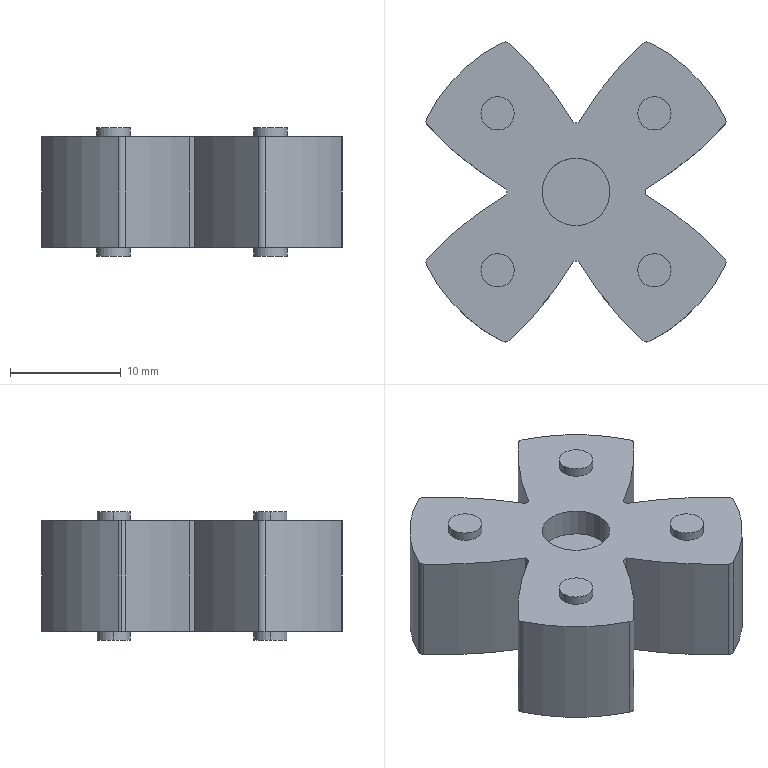Part | STEP file | BODY2_E-LMPJC30L35-14-15-LK5 | 1 solid | 59 faces | box 27.051 x 27.051 x 11.6 mm | volume 4769 mm3 | cylinder 47 | plane 12 | commonest cylinder face diameters 3 x16 1 x10 61.94 x8 12.5 x5 6.1 x4 30 x4